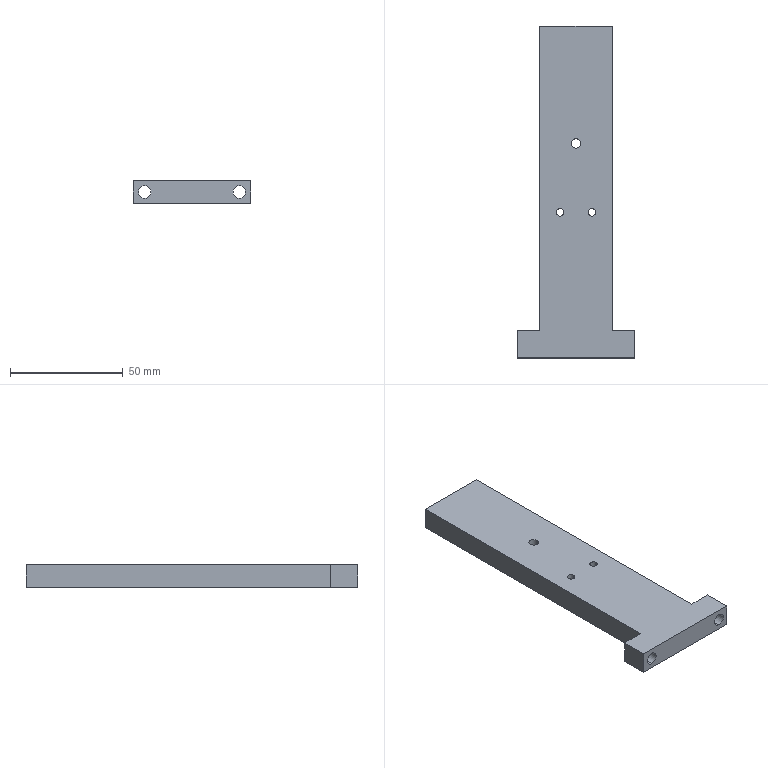Part | STEP file | B05 | 1 solid | 28 faces | box 52 x 147 x 10 mm | volume 48382 mm3 | cylinder 14 | plane 10 | cone 4 | commonest cylinder face diameters 3.3 x8 5.5 x4 4.2 x2